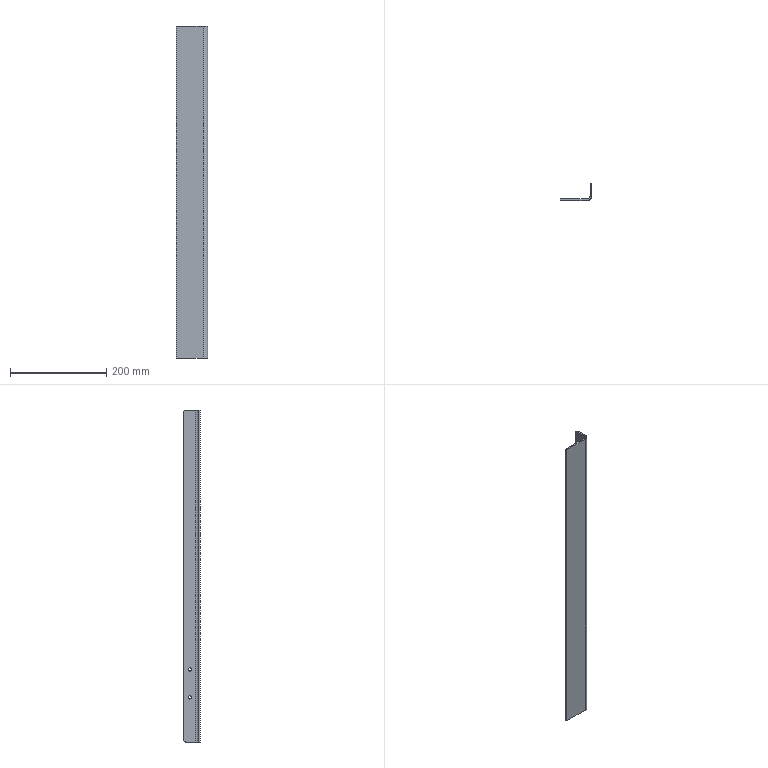Part | SolidWorks | features Fillet 1, FlatPattern 1, ICE 1, SMBaseFlange 1, SheetMetal 1 | 1 solid | 20 faces | box 65 x 35 x 690 mm | volume 206237 mm3 | plane 12 | cylinder 8 | commonest cylinder face diameters 7.2 x4 10 x2 12 x1 18.4 x1
STEP:
#1=CARTESIAN_POINT('',(-3.2,22.,-197.7));
#2=VERTEX_POINT('',#1);
#3=CARTESIAN_POINT('',(-3.2,22.,-190.5));
#4=VERTEX_POINT('',#3);
#5=CARTESIAN_POINT('',(-3.2,22.,-194.1));
#6=DIRECTION('',(-1.,0.,0.));
#7=DIRECTION('',(0.,0.,1.));
#8=AXIS2_PLACEMENT_3D('',#5,#6,#7);
#9=CIRCLE('',#8,3.6);
#10=EDGE_CURVE('',#2,#4,#9,.T.);
#11=ORIENTED_EDGE('',*,*,#10,.T.);
#12=CARTESIAN_POINT('',(0.,22.,-190.5));
#13=VERTEX_POINT('',#12);
#14=CARTESIAN_POINT('',(-65.,22.,-190.5));
#15=DIRECTION('',(1.,0.,0.));
#16=VECTOR('',#15,1000.);
#17=LINE('',#14,#16);
#18=EDGE_CURVE('',#4,#13,#17,.T.);
#19=ORIENTED_EDGE('',*,*,#18,.T.);
#20=CARTESIAN_POINT('',(0.,22.,-197.7));
#21=VERTEX_POINT('',#20);
#22=CARTESIAN_POINT('',(0.,22.,-194.1));
#23=DIRECTION('',(1.,0.,0.));
#24=DIRECTION('',(0.,0.,-1.));
#25=AXIS2_PLACEMENT_3D('',#22,#23,#24);
#26=CIRCLE('',#25,3.6);
#27=EDGE_CURVE('',#13,#21,#26,.T.);
#28=ORIENTED_EDGE('',*,*,#27,.T.);
#29=CARTESIAN_POINT('',(-65.,22.,-197.7));
#30=DIRECTION('',(1.,0.,0.));
#31=VECTOR('',#30,1000.);
#32=LINE('',#29,#31);
#33=EDGE_CURVE('',#2,#21,#32,.T.);
#34=ORIENTED_EDGE('',*,*,#33,.F.);
#35=EDGE_LOOP('',(#11,#19,#28,#34));
#36=FACE_OUTER_BOUND('',#35,.T.);
#37=CARTESIAN_POINT('',(-65.,22.,-194.1));
#38=DIRECTION('',(1.,0.,0.));
#39=DIRECTION('',(0.,0.,-1.));
#40=AXIS2_PLACEMENT_3D('',#37,#38,#39);
#41=CYLINDRICAL_SURFACE('',#40,3.6);
#42=ADVANCED_FACE('',(#36),#41,.F.);
#43=CARTESIAN_POINT('',(-3.2,22.,-255.7));
#44=VERTEX_POINT('',#43);
#45=CARTESIAN_POINT('',(-3.2,22.,-248.5));
#46=VERTEX_POINT('',#45);
#47=CARTESIAN_POINT('',(-3.2,22.,-252.1));
#48=DIRECTION('',(-1.,0.,0.));
#49=DIRECTION('',(0.,0.,1.));
#50=AXIS2_PLACEMENT_3D('',#47,#48,#49);
#51=CIRCLE('',#50,3.6);
#52=EDGE_CURVE('',#44,#46,#51,.T.);
#53=ORIENTED_EDGE('',*,*,#52,.T.);
#54=CARTESIAN_POINT('',(0.,22.,-248.5));
#55=VERTEX_POINT('',#54);
#56=CARTESIAN_POINT('',(-65.,22.,-248.5));
#57=DIRECTION('',(1.,0.,0.));
#58=VECTOR('',#57,1000.);
#59=LINE('',#56,#58);
#60=EDGE_CURVE('',#46,#55,#59,.T.);
#61=ORIENTED_EDGE('',*,*,#60,.T.);
#62=CARTESIAN_POINT('',(0.,22.,-255.7));
#63=VERTEX_POINT('',#62);
#64=CARTESIAN_POINT('',(0.,22.,-252.1));
#65=DIRECTION('',(1.,0.,0.));
#66=DIRECTION('',(0.,0.,-1.));
#67=AXIS2_PLACEMENT_3D('',#64,#65,#66);
#68=CIRCLE('',#67,3.6);
#69=EDGE_CURVE('',#55,#63,#68,.T.);
#70=ORIENTED_EDGE('',*,*,#69,.T.);
#71=CARTESIAN_POINT('',(-65.,22.,-255.7));
#72=DIRECTION('',(1.,0.,0.));
#73=VECTOR('',#72,1000.);
#74=LINE('',#71,#73);
#75=EDGE_CURVE('',#44,#63,#74,.T.);
#76=ORIENTED_EDGE('',*,*,#75,.F.);
#77=EDGE_LOOP('',(#53,#61,#70,#76));
#78=FACE_OUTER_BOUND('',#77,.T.);
#79=CARTESIAN_POINT('',(-65.,22.,-252.1));
#80=DIRECTION('',(1.,0.,0.));
#81=DIRECTION('',(0.,0.,-1.));
#82=AXIS2_PLACEMENT_3D('',#79,#80,#81);
#83=CYLINDRICAL_SURFACE('',#82,3.6);
#84=ADVANCED_FACE('',(#78),#83,.F.);
#85=CARTESIAN_POINT('',(-9.2,0.,345.));
#86=VERTEX_POINT('',#85);
#87=CARTESIAN_POINT('',(-9.2,3.2,345.));
#88=VERTEX_POINT('',#87);
#89=CARTESIAN_POINT('',(-9.2,0.,345.));
#90=DIRECTION('',(0.,1.,0.));
#91=VECTOR('',#90,1000.);
#92=LINE('',#89,#91);
#93=EDGE_CURVE('',#86,#88,#92,.T.);
#94=ORIENTED_EDGE('',*,*,#93,.F.);
#95=CARTESIAN_POINT('',(0.,9.2,345.));
#96=VERTEX_POINT('',#95);
#97=CARTESIAN_POINT('',(-9.2,9.2,345.));
#98=DIRECTION('',(0.,0.,1.));
#99=DIRECTION('',(-1.,0.,0.));
#100=AXIS2_PLACEMENT_3D('',#97,#98,#99);
#101=CIRCLE('',#100,9.2);
#102=EDGE_CURVE('',#86,#96,#101,.T.);
#103=ORIENTED_EDGE('',*,*,#102,.T.);
#104=CARTESIAN_POINT('',(-3.2,9.2,345.));
#105=VERTEX_POINT('',#104);
#106=CARTESIAN_POINT('',(-3.2,9.2,345.));
#107=DIRECTION('',(1.,0.,0.));
#108=VECTOR('',#107,1000.);
#109=LINE('',#106,#108);
#110=EDGE_CURVE('',#105,#96,#109,.T.);
#111=ORIENTED_EDGE('',*,*,#110,.F.);
#112=CARTESIAN_POINT('',(-9.2,9.2,345.));
#113=DIRECTION('',(0.,0.,1.));
#114=DIRECTION('',(1.,0.,0.));
#115=AXIS2_PLACEMENT_3D('',#112,#113,#114);
#116=CIRCLE('',#115,6.);
#117=EDGE_CURVE('',#88,#105,#116,.T.);
#118=ORIENTED_EDGE('',*,*,#117,.F.);
#119=EDGE_LOOP('',(#94,#103,#111,#118));
#120=FACE_OUTER_BOUND('',#119,.T.);
#121=CARTESIAN_POINT('',(-9.2,0.,345.));
#122=DIRECTION('',(0.,0.,1.));
#123=DIRECTION('',(1.,0.,0.));
#124=AXIS2_PLACEMENT_3D('',#121,#122,#123);
#125=PLANE('',#124);
#126=ADVANCED_FACE('',(#120),#125,.T.);
#127=CARTESIAN_POINT('',(-65.,0.,345.));
#128=VERTEX_POINT('',#127);
#129=CARTESIAN_POINT('',(0.,0.,345.));
#130=DIRECTION('',(1.,0.,0.));
#131=VECTOR('',#130,1000.);
#132=LINE('',#129,#131);
#133=EDGE_CURVE('',#128,#86,#132,.T.);
#134=ORIENTED_EDGE('',*,*,#133,.T.);
#135=ORIENTED_EDGE('',*,*,#93,.T.);
#136=CARTESIAN_POINT('',(-65.,3.2,345.));
#137=VERTEX_POINT('',#136);
#138=CARTESIAN_POINT('',(0.,3.2,345.));
#139=DIRECTION('',(1.,0.,0.));
#140=VECTOR('',#139,1000.);
#141=LINE('',#138,#140);
#142=EDGE_CURVE('',#137,#88,#141,.T.);
#143=ORIENTED_EDGE('',*,*,#142,.F.);
#144=CARTESIAN_POINT('',(-65.,0.,345.));
#145=DIRECTION('',(0.,1.,0.));
#146=VECTOR('',#145,1000.);
#147=LINE('',#144,#146);
#148=EDGE_CURVE('',#128,#137,#147,.T.);
#149=ORIENTED_EDGE('',*,*,#148,.F.);
#150=EDGE_LOOP('',(#134,#135,#143,#149));
#151=FACE_OUTER_BOUND('',#150,.T.);
#152=CARTESIAN_POINT('',(-3.2,9.2,345.));
#153=DIRECTION('',(0.,0.,1.));
#154=DIRECTION('',(1.,0.,0.));
#155=AXIS2_PLACEMENT_3D('',#152,#153,#154);
#156=PLANE('',#155);
#157=ADVANCED_FACE('',(#151),#156,.T.);
#158=CARTESIAN_POINT('',(0.,9.2,-345.));
#159=VERTEX_POINT('',#158);
#160=CARTESIAN_POINT('',(-3.2,9.2,-345.));
#161=VERTEX_POINT('',#160);
#162=CARTESIAN_POINT('',(0.,9.2,-345.));
#163=DIRECTION('',(-1.,0.,0.));
#164=VECTOR('',#163,1000.);
#165=LINE('',#162,#164);
#166=EDGE_CURVE('',#159,#161,#165,.T.);
#167=ORIENTED_EDGE('',*,*,#166,.F.);
#168=CARTESIAN_POINT('',(-9.2,0.,-345.));
#169=VERTEX_POINT('',#168);
#170=CARTESIAN_POINT('',(-9.2,9.2,-345.));
#171=DIRECTION('',(0.,0.,1.));
#172=DIRECTION('',(-1.,0.,0.));
#173=AXIS2_PLACEMENT_3D('',#170,#171,#172);
#174=CIRCLE('',#173,9.2);
#175=EDGE_CURVE('',#169,#159,#174,.T.);
#176=ORIENTED_EDGE('',*,*,#175,.F.);
#177=CARTESIAN_POINT('',(-9.2,3.2,-345.));
#178=VERTEX_POINT('',#177);
#179=CARTESIAN_POINT('',(-9.2,3.2,-345.));
#180=DIRECTION('',(0.,-1.,0.));
#181=VECTOR('',#180,1000.);
#182=LINE('',#179,#181);
#183=EDGE_CURVE('',#178,#169,#182,.T.);
#184=ORIENTED_EDGE('',*,*,#183,.F.);
#185=CARTESIAN_POINT('',(-9.2,9.2,-345.));
#186=DIRECTION('',(0.,0.,1.));
#187=DIRECTION('',(1.,0.,0.));
#188=AXIS2_PLACEMENT_3D('',#185,#186,#187);
#189=CIRCLE('',#188,6.);
#190=EDGE_CURVE('',#178,#161,#189,.T.);
#191=ORIENTED_EDGE('',*,*,#190,.T.);
#192=EDGE_LOOP('',(#167,#176,#184,#191));
#193=FACE_OUTER_BOUND('',#192,.T.);
#194=CARTESIAN_POINT('',(0.,9.2,-345.));
#195=DIRECTION('',(0.,0.,-1.));
#196=DIRECTION('',(-1.,0.,0.));
#197=AXIS2_PLACEMENT_3D('',#194,#195,#196);
#198=PLANE('',#197);
#199=ADVANCED_FACE('',(#193),#198,.T.);
#200=CARTESIAN_POINT('',(-3.2,30.,-345.));
#201=VERTEX_POINT('',#200);
#202=CARTESIAN_POINT('',(-3.2,0.,-345.));
#203=DIRECTION('',(0.,1.,0.));
#204=VECTOR('',#203,1000.);
#205=LINE('',#202,#204);
#206=EDGE_CURVE('',#161,#201,#205,.T.);
#207=ORIENTED_EDGE('',*,*,#206,.T.);
#208=CARTESIAN_POINT('',(0.,30.,-345.));
#209=VERTEX_POINT('',#208);
#210=CARTESIAN_POINT('',(-9.2,30.,-345.));
#211=DIRECTION('',(1.,0.,0.));
#212=VECTOR('',#211,1000.);
#213=LINE('',#210,#212);
#214=EDGE_CURVE('',#201,#209,#213,.T.);
#215=ORIENTED_EDGE('',*,*,#214,.T.);
#216=CARTESIAN_POINT('',(0.,0.,-345.));
#217=DIRECTION('',(0.,1.,0.));
#218=VECTOR('',#217,1000.);
#219=LINE('',#216,#218);
#220=EDGE_CURVE('',#159,#209,#219,.T.);
#221=ORIENTED_EDGE('',*,*,#220,.F.);
#222=ORIENTED_EDGE('',*,*,#166,.T.);
#223=EDGE_LOOP('',(#207,#215,#221,#222));
#224=FACE_OUTER_BOUND('',#223,.T.);
#225=CARTESIAN_POINT('',(-9.2,3.2,-345.));
#226=DIRECTION('',(0.,0.,-1.));
#227=DIRECTION('',(-1.,0.,0.));
#228=AXIS2_PLACEMENT_3D('',#225,#226,#227);
#229=PLANE('',#228);
#230=ADVANCED_FACE('',(#224),#229,.T.);
#231=CARTESIAN_POINT('',(0.,22.,-194.1));
#232=DIRECTION('',(1.,0.,0.));
#233=DIRECTION('',(0.,0.,-1.));
#234=AXIS2_PLACEMENT_3D('',#231,#232,#233);
#235=CIRCLE('',#234,3.6);
#236=EDGE_CURVE('',#21,#13,#235,.T.);
#237=ORIENTED_EDGE('',*,*,#236,.F.);
#238=ORIENTED_EDGE('',*,*,#27,.F.);
#239=EDGE_LOOP('',(#237,#238));
#240=FACE_BOUND('',#239,.T.);
#241=CARTESIAN_POINT('',(0.,22.,-252.1));
#242=DIRECTION('',(1.,0.,0.));
#243=DIRECTION('',(0.,0.,-1.));
#244=AXIS2_PLACEMENT_3D('',#241,#242,#243);
#245=CIRCLE('',#244,3.6);
#246=EDGE_CURVE('',#63,#55,#245,.T.);
#247=ORIENTED_EDGE('',*,*,#246,.F.);
#248=ORIENTED_EDGE('',*,*,#69,.F.);
#249=EDGE_LOOP('',(#247,#248));
#250=FACE_BOUND('',#249,.T.);
#251=CARTESIAN_POINT('',(0.,35.,340.));
#252=VERTEX_POINT('',#251);
#253=CARTESIAN_POINT('',(0.,35.,-340.));
#254=VERTEX_POINT('',#253);
#255=CARTESIAN_POINT('',(0.,35.,345.));
#256=DIRECTION('',(0.,0.,-1.));
#257=VECTOR('',#256,1000.);
#258=LINE('',#255,#257);
#259=EDGE_CURVE('',#252,#254,#258,.T.);
#260=ORIENTED_EDGE('',*,*,#259,.F.);
#261=CARTESIAN_POINT('',(0.,30.,345.));
#262=VERTEX_POINT('',#261);
#263=CARTESIAN_POINT('',(0.,30.,340.));
#264=DIRECTION('',(1.,0.,0.));
#265=DIRECTION('',(0.,0.,1.));
#266=AXIS2_PLACEMENT_3D('',#263,#264,#265);
#267=CIRCLE('',#266,5.);
#268=EDGE_CURVE('',#252,#262,#267,.T.);
#269=ORIENTED_EDGE('',*,*,#268,.T.);
#270=CARTESIAN_POINT('',(0.,0.,345.));
#271=DIRECTION('',(0.,1.,0.));
#272=VECTOR('',#271,1000.);
#273=LINE('',#270,#272);
#274=EDGE_CURVE('',#96,#262,#273,.T.);
#275=ORIENTED_EDGE('',*,*,#274,.F.);
#276=CARTESIAN_POINT('',(0.,9.2,345.));
#277=DIRECTION('',(0.,0.,-1.));
#278=VECTOR('',#277,1000.);
#279=LINE('',#276,#278);
#280=EDGE_CURVE('',#96,#159,#279,.T.);
#281=ORIENTED_EDGE('',*,*,#280,.T.);
#282=ORIENTED_EDGE('',*,*,#220,.T.);
#283=CARTESIAN_POINT('',(0.,30.,-340.));
#284=DIRECTION('',(1.,0.,0.));
#285=DIRECTION('',(0.,0.,1.));
#286=AXIS2_PLACEMENT_3D('',#283,#284,#285);
#287=CIRCLE('',#286,5.);
#288=EDGE_CURVE('',#209,#254,#287,.T.);
#289=ORIENTED_EDGE('',*,*,#288,.T.);
#290=EDGE_LOOP('',(#260,#269,#275,#281,#282,#289));
#291=FACE_OUTER_BOUND('',#290,.T.);
#292=CARTESIAN_POINT('',(0.,0.,345.));
#293=DIRECTION('',(-1.,0.,0.));
#294=DIRECTION('',(0.,0.,1.));
#295=AXIS2_PLACEMENT_3D('',#292,#293,#294);
#296=PLANE('',#295);
#297=ADVANCED_FACE('',(#240,#250,#291),#296,.F.);
#298=CARTESIAN_POINT('',(-3.2,35.,340.));
#299=VERTEX_POINT('',#298);
#300=CARTESIAN_POINT('',(-3.2,35.,-340.));
#301=VERTEX_POINT('',#300);
#302=CARTESIAN_POINT('',(-3.2,35.,345.));
#303=DIRECTION('',(0.,0.,-1.));
#304=VECTOR('',#303,1000.);
#305=LINE('',#302,#304);
#306=EDGE_CURVE('',#299,#301,#305,.T.);
#307=ORIENTED_EDGE('',*,*,#306,.F.);
#308=CARTESIAN_POINT('',(-3.2,35.,340.));
#309=DIRECTION('',(1.,0.,0.));
#310=VECTOR('',#309,1000.);
#311=LINE('',#308,#310);
#312=EDGE_CURVE('',#299,#252,#311,.T.);
#313=ORIENTED_EDGE('',*,*,#312,.T.);
#314=ORIENTED_EDGE('',*,*,#259,.T.);
#315=CARTESIAN_POINT('',(-3.2,35.,-340.));
#316=DIRECTION('',(-1.,0.,0.));
#317=VECTOR('',#316,1000.);
#318=LINE('',#315,#317);
#319=EDGE_CURVE('',#254,#301,#318,.T.);
#320=ORIENTED_EDGE('',*,*,#319,.T.);
#321=EDGE_LOOP('',(#307,#313,#314,#320));
#322=FACE_OUTER_BOUND('',#321,.T.);
#323=CARTESIAN_POINT('',(-3.2,35.,345.));
#324=DIRECTION('',(0.,1.,0.));
#325=DIRECTION('',(0.,0.,1.));
#326=AXIS2_PLACEMENT_3D('',#323,#324,#325);
#327=PLANE('',#326);
#328=ADVANCED_FACE('',(#322),#327,.T.);
#329=ORIENTED_EDGE('',*,*,#10,.F.);
#330=CARTESIAN_POINT('',(-3.2,22.,-194.1));
#331=DIRECTION('',(-1.,0.,0.));
#332=DIRECTION('',(0.,0.,1.));
#333=AXIS2_PLACEMENT_3D('',#330,#331,#332);
#334=CIRCLE('',#333,3.6);
#335=EDGE_CURVE('',#4,#2,#334,.T.);
#336=ORIENTED_EDGE('',*,*,#335,.F.);
#337=EDGE_LOOP('',(#329,#336));
#338=FACE_BOUND('',#337,.T.);
#339=ORIENTED_EDGE('',*,*,#52,.F.);
#340=CARTESIAN_POINT('',(-3.2,22.,-252.1));
#341=DIRECTION('',(-1.,0.,0.));
#342=DIRECTION('',(0.,0.,1.));
#343=AXIS2_PLACEMENT_3D('',#340,#341,#342);
#344=CIRCLE('',#343,3.6);
#345=EDGE_CURVE('',#46,#44,#344,.T.);
#346=ORIENTED_EDGE('',*,*,#345,.F.);
#347=EDGE_LOOP('',(#339,#346));
#348=FACE_BOUND('',#347,.T.);
#349=CARTESIAN_POINT('',(-3.2,30.,345.));
#350=VERTEX_POINT('',#349);
#351=CARTESIAN_POINT('',(-3.2,0.,345.));
#352=DIRECTION('',(0.,1.,0.));
#353=VECTOR('',#352,1000.);
#354=LINE('',#351,#353);
#355=EDGE_CURVE('',#105,#350,#354,.T.);
#356=ORIENTED_EDGE('',*,*,#355,.T.);
#357=CARTESIAN_POINT('',(-3.2,30.,340.));
#358=DIRECTION('',(-1.,0.,0.));
#359=DIRECTION('',(0.,0.,1.));
#360=AXIS2_PLACEMENT_3D('',#357,#358,#359);
#361=CIRCLE('',#360,5.);
#362=EDGE_CURVE('',#350,#299,#361,.T.);
#363=ORIENTED_EDGE('',*,*,#362,.T.);
#364=ORIENTED_EDGE('',*,*,#306,.T.);
#365=CARTESIAN_POINT('',(-3.2,30.,-340.));
#366=DIRECTION('',(-1.,0.,0.));
#367=DIRECTION('',(0.,0.,1.));
#368=AXIS2_PLACEMENT_3D('',#365,#366,#367);
#369=CIRCLE('',#368,5.);
#370=EDGE_CURVE('',#301,#201,#369,.T.);
#371=ORIENTED_EDGE('',*,*,#370,.T.);
#372=ORIENTED_EDGE('',*,*,#206,.F.);
#373=CARTESIAN_POINT('',(-3.2,9.2,345.));
#374=DIRECTION('',(0.,0.,-1.));
#375=VECTOR('',#374,1000.);
#376=LINE('',#373,#375);
#377=EDGE_CURVE('',#105,#161,#376,.T.);
#378=ORIENTED_EDGE('',*,*,#377,.F.);
#379=EDGE_LOOP('',(#356,#363,#364,#371,#372,#378));
#380=FACE_OUTER_BOUND('',#379,.T.);
#381=CARTESIAN_POINT('',(-3.2,0.,345.));
#382=DIRECTION('',(-1.,0.,0.));
#383=DIRECTION('',(0.,0.,1.));
#384=AXIS2_PLACEMENT_3D('',#381,#382,#383);
#385=PLANE('',#384);
#386=ADVANCED_FACE('',(#338,#348,#380),#385,.T.);
#387=ORIENTED_EDGE('',*,*,#190,.F.);
#388=CARTESIAN_POINT('',(-9.2,3.2,345.));
#389=DIRECTION('',(0.,0.,-1.));
#390=VECTOR('',#389,1000.);
#391=LINE('',#388,#390);
#392=EDGE_CURVE('',#88,#178,#391,.T.);
#393=ORIENTED_EDGE('',*,*,#392,.F.);
#394=ORIENTED_EDGE('',*,*,#117,.T.);
#395=ORIENTED_EDGE('',*,*,#377,.T.);
#396=EDGE_LOOP('',(#387,#393,#394,#395));
#397=FACE_OUTER_BOUND('',#396,.T.);
#398=CARTESIAN_POINT('',(-9.2,9.2,345.));
#399=DIRECTION('',(0.,0.,-1.));
#400=DIRECTION('',(-1.,0.,0.));
#401=AXIS2_PLACEMENT_3D('',#398,#399,#400);
#402=CYLINDRICAL_SURFACE('',#401,6.);
#403=ADVANCED_FACE('',(#397),#402,.F.);
#404=CARTESIAN_POINT('',(-65.,3.2,-345.));
#405=VERTEX_POINT('',#404);
#406=CARTESIAN_POINT('',(0.,3.2,-345.));
#407=DIRECTION('',(1.,0.,0.));
#408=VECTOR('',#407,1000.);
#409=LINE('',#406,#408);
#410=EDGE_CURVE('',#405,#178,#409,.T.);
#411=ORIENTED_EDGE('',*,*,#410,.F.);
#412=CARTESIAN_POINT('',(-65.,3.2,345.));
#413=DIRECTION('',(0.,0.,-1.));
#414=VECTOR('',#413,1000.);
#415=LINE('',#412,#414);
#416=EDGE_CURVE('',#137,#405,#415,.T.);
#417=ORIENTED_EDGE('',*,*,#416,.F.);
#418=ORIENTED_EDGE('',*,*,#142,.T.);
#419=ORIENTED_EDGE('',*,*,#392,.T.);
#420=EDGE_LOOP('',(#411,#417,#418,#419));
#421=FACE_OUTER_BOUND('',#420,.T.);
#422=CARTESIAN_POINT('',(0.,3.2,345.));
#423=DIRECTION('',(0.,1.,0.));
#424=DIRECTION('',(0.,0.,1.));
#425=AXIS2_PLACEMENT_3D('',#422,#423,#424);
#426=PLANE('',#425);
#427=ADVANCED_FACE('',(#421),#426,.T.);
#428=CARTESIAN_POINT('',(-65.,0.,-345.));
#429=VERTEX_POINT('',#428);
#430=CARTESIAN_POINT('',(-65.,0.,-345.));
#431=DIRECTION('',(0.,1.,0.));
#432=VECTOR('',#431,1000.);
#433=LINE('',#430,#432);
#434=EDGE_CURVE('',#429,#405,#433,.T.);
#435=ORIENTED_EDGE('',*,*,#434,.F.);
#436=CARTESIAN_POINT('',(-65.,0.,345.));
#437=DIRECTION('',(0.,0.,-1.));
#438=VECTOR('',#437,1000.);
#439=LINE('',#436,#438);
#440=EDGE_CURVE('',#128,#429,#439,.T.);
#441=ORIENTED_EDGE('',*,*,#440,.F.);
#442=ORIENTED_EDGE('',*,*,#148,.T.);
#443=ORIENTED_EDGE('',*,*,#416,.T.);
#444=EDGE_LOOP('',(#435,#441,#442,#443));
#445=FACE_OUTER_BOUND('',#444,.T.);
#446=CARTESIAN_POINT('',(-65.,0.,345.));
#447=DIRECTION('',(-1.,0.,0.));
#448=DIRECTION('',(0.,0.,1.));
#449=AXIS2_PLACEMENT_3D('',#446,#447,#448);
#450=PLANE('',#449);
#451=ADVANCED_FACE('',(#445),#450,.T.);
#452=CARTESIAN_POINT('',(0.,0.,-345.));
#453=DIRECTION('',(1.,0.,0.));
#454=VECTOR('',#453,1000.);
#455=LINE('',#452,#454);
#456=EDGE_CURVE('',#429,#169,#455,.T.);
#457=ORIENTED_EDGE('',*,*,#456,.T.);
#458=CARTESIAN_POINT('',(-9.2,0.,345.));
#459=DIRECTION('',(0.,0.,-1.));
#460=VECTOR('',#459,1000.);
#461=LINE('',#458,#460);
#462=EDGE_CURVE('',#86,#169,#461,.T.);
#463=ORIENTED_EDGE('',*,*,#462,.F.);
#464=ORIENTED_EDGE('',*,*,#133,.F.);
#465=ORIENTED_EDGE('',*,*,#440,.T.);
#466=EDGE_LOOP('',(#457,#463,#464,#465));
#467=FACE_OUTER_BOUND('',#466,.T.);
#468=CARTESIAN_POINT('',(0.,0.,345.));
#469=DIRECTION('',(0.,1.,0.));
#470=DIRECTION('',(0.,0.,1.));
#471=AXIS2_PLACEMENT_3D('',#468,#469,#470);
#472=PLANE('',#471);
#473=ADVANCED_FACE('',(#467),#472,.F.);
#474=ORIENTED_EDGE('',*,*,#175,.T.);
#475=ORIENTED_EDGE('',*,*,#280,.F.);
#476=ORIENTED_EDGE('',*,*,#102,.F.);
#477=ORIENTED_EDGE('',*,*,#462,.T.);
#478=EDGE_LOOP('',(#474,#475,#476,#477));
#479=FACE_OUTER_BOUND('',#478,.T.);
#480=CARTESIAN_POINT('',(-9.2,9.2,345.));
#481=DIRECTION('',(0.,0.,-1.));
#482=DIRECTION('',(-1.,0.,0.));
#483=AXIS2_PLACEMENT_3D('',#480,#481,#482);
#484=CYLINDRICAL_SURFACE('',#483,9.2);
#485=ADVANCED_FACE('',(#479),#484,.T.);
#486=ORIENTED_EDGE('',*,*,#274,.T.);
#487=CARTESIAN_POINT('',(-9.2,30.,345.));
#488=DIRECTION('',(-1.,0.,0.));
#489=VECTOR('',#488,1000.);
#490=LINE('',#487,#489);
#491=EDGE_CURVE('',#262,#350,#490,.T.);
#492=ORIENTED_EDGE('',*,*,#491,.T.);
#493=ORIENTED_EDGE('',*,*,#355,.F.);
#494=ORIENTED_EDGE('',*,*,#110,.T.);
#495=EDGE_LOOP('',(#486,#492,#493,#494));
#496=FACE_OUTER_BOUND('',#495,.T.);
#497=CARTESIAN_POINT('',(-9.2,9.2,345.));
#498=DIRECTION('',(0.,0.,1.));
#499=DIRECTION('',(1.,0.,0.));
#500=AXIS2_PLACEMENT_3D('',#497,#498,#499);
#501=PLANE('',#500);
#502=ADVANCED_FACE('',(#496),#501,.T.);
#503=ORIENTED_EDGE('',*,*,#410,.T.);
#504=ORIENTED_EDGE('',*,*,#183,.T.);
#505=ORIENTED_EDGE('',*,*,#456,.F.);
#506=ORIENTED_EDGE('',*,*,#434,.T.);
#507=EDGE_LOOP('',(#503,#504,#505,#506));
#508=FACE_OUTER_BOUND('',#507,.T.);
#509=CARTESIAN_POINT('',(-9.2,9.2,-345.));
#510=DIRECTION('',(0.,0.,1.));
#511=DIRECTION('',(1.,0.,0.));
#512=AXIS2_PLACEMENT_3D('',#509,#510,#511);
#513=PLANE('',#512);
#514=ADVANCED_FACE('',(#508),#513,.F.);
#515=ORIENTED_EDGE('',*,*,#60,.F.);
#516=ORIENTED_EDGE('',*,*,#345,.T.);
#517=ORIENTED_EDGE('',*,*,#75,.T.);
#518=ORIENTED_EDGE('',*,*,#246,.T.);
#519=EDGE_LOOP('',(#515,#516,#517,#518));
#520=FACE_OUTER_BOUND('',#519,.T.);
#521=CARTESIAN_POINT('',(-65.,22.,-252.1));
#522=DIRECTION('',(1.,0.,0.));
#523=DIRECTION('',(0.,0.,-1.));
#524=AXIS2_PLACEMENT_3D('',#521,#522,#523);
#525=CYLINDRICAL_SURFACE('',#524,3.6);
#526=ADVANCED_FACE('',(#520),#525,.F.);
#527=ORIENTED_EDGE('',*,*,#18,.F.);
#528=ORIENTED_EDGE('',*,*,#335,.T.);
#529=ORIENTED_EDGE('',*,*,#33,.T.);
#530=ORIENTED_EDGE('',*,*,#236,.T.);
#531=EDGE_LOOP('',(#527,#528,#529,#530));
#532=FACE_OUTER_BOUND('',#531,.T.);
#533=CARTESIAN_POINT('',(-65.,22.,-194.1));
#534=DIRECTION('',(1.,0.,0.));
#535=DIRECTION('',(0.,0.,-1.));
#536=AXIS2_PLACEMENT_3D('',#533,#534,#535);
#537=CYLINDRICAL_SURFACE('',#536,3.6);
#538=ADVANCED_FACE('',(#532),#537,.F.);
#539=ORIENTED_EDGE('',*,*,#362,.F.);
#540=ORIENTED_EDGE('',*,*,#491,.F.);
#541=ORIENTED_EDGE('',*,*,#268,.F.);
#542=ORIENTED_EDGE('',*,*,#312,.F.);
#543=EDGE_LOOP('',(#539,#540,#541,#542));
#544=FACE_OUTER_BOUND('',#543,.T.);
#545=CARTESIAN_POINT('',(-3.2,30.,340.));
#546=DIRECTION('',(1.,0.,0.));
#547=DIRECTION('',(0.,0.,-1.));
#548=AXIS2_PLACEMENT_3D('',#545,#546,#547);
#549=CYLINDRICAL_SURFACE('',#548,5.);
#550=ADVANCED_FACE('',(#544),#549,.T.);
#551=ORIENTED_EDGE('',*,*,#370,.F.);
#552=ORIENTED_EDGE('',*,*,#319,.F.);
#553=ORIENTED_EDGE('',*,*,#288,.F.);
#554=ORIENTED_EDGE('',*,*,#214,.F.);
#555=EDGE_LOOP('',(#551,#552,#553,#554));
#556=FACE_OUTER_BOUND('',#555,.T.);
#557=CARTESIAN_POINT('',(-9.2,30.,-340.));
#558=DIRECTION('',(1.,0.,0.));
#559=DIRECTION('',(0.,0.,-1.));
#560=AXIS2_PLACEMENT_3D('',#557,#558,#559);
#561=CYLINDRICAL_SURFACE('',#560,5.);
#562=ADVANCED_FACE('',(#556),#561,.T.);
#563=CLOSED_SHELL('',(#42,#84,#126,#157,#199,#230,#297,#328,#386,#403,#427,#451,#473,#485,#502,#514,#526,#538,#550,#562));
#564=MANIFOLD_SOLID_BREP('',#563);
#565=CARTESIAN_POINT('',(0.,0.,0.));
#566=DIRECTION('',(0.,0.,1.));
#567=DIRECTION('',(1.,0.,0.));
#568=AXIS2_PLACEMENT_3D('',#565,#566,#567);
#569=(LENGTH_UNIT()NAMED_UNIT(*)SI_UNIT(.MILLI.,.METRE.));
#570=UNCERTAINTY_MEASURE_WITH_UNIT(LENGTH_MEASURE(0.00001),#569,'','');
#571=(NAMED_UNIT(*)PLANE_ANGLE_UNIT()SI_UNIT($,.RADIAN.));
#572=(NAMED_UNIT(*)SI_UNIT($,.STERADIAN.)SOLID_ANGLE_UNIT());
#573=(GEOMETRIC_REPRESENTATION_CONTEXT(3)GLOBAL_UNCERTAINTY_ASSIGNED_CONTEXT((#570))GLOBAL_UNIT_ASSIGNED_CONTEXT((#569,#571,#572))REPRESENTATION_CONTEXT('',''));
#574=ADVANCED_BREP_SHAPE_REPRESENTATION('',(#564,#568),#573);